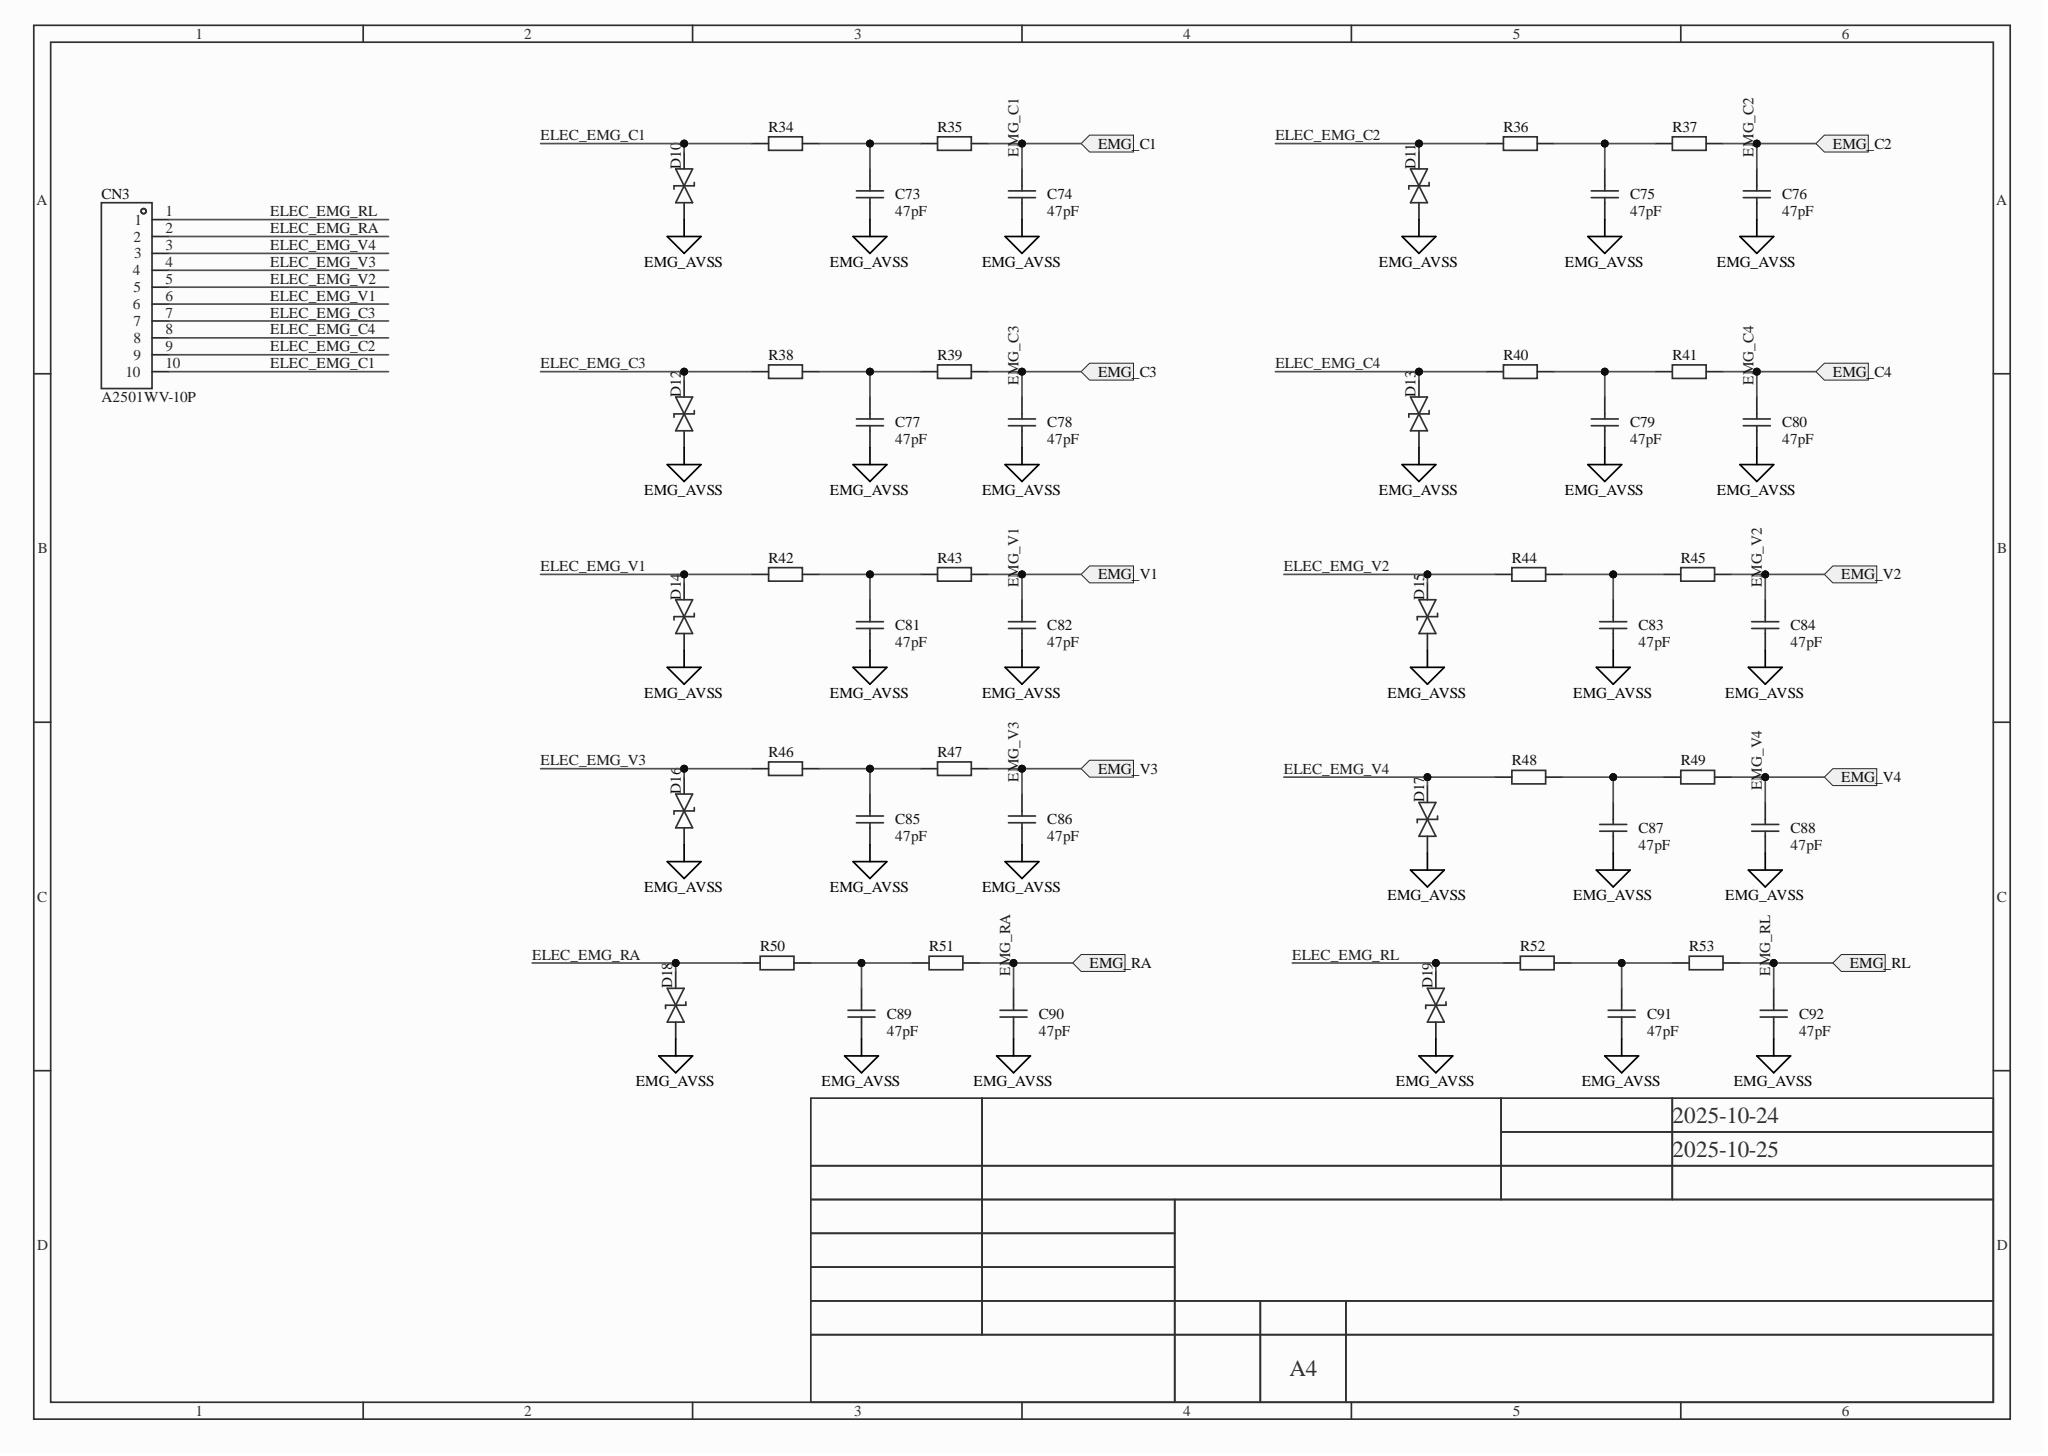Circuit board | Altium Designer | 212 parts | 123 nets | one sheet of the schematic
Parts on this sheet (reference | value | footprint):
C73 | 47pF | C0402
C74 | 47pF | C0402
C75 | 47pF | C0402
C76 | 47pF | C0402
C77 | 47pF | C0402
C78 | 47pF | C0402
C79 | 47pF | C0402
C80 | 47pF | C0402
C81 | 47pF | C0402
C82 | 47pF | C0402
C83 | 47pF | C0402
C84 | 47pF | C0402
C85 | 47pF | C0402
C86 | 47pF | C0402
C87 | 47pF | C0402
C88 | 47pF | C0402
C89 | 47pF | C0402
C90 | 47pF | C0402
C91 | 47pF | C0402
C92 | 47pF | C0402
CN3 | A2501WV-10P | CONN-TH_A2501WV-10P
D10 | TPD1E10B06DPYR-TP | X1-DFN1006-2_L1.0-W0.6-BI
D11 | TPD1E10B06DPYR-TP | X1-DFN1006-2_L1.0-W0.6-BI
D12 | TPD1E10B06DPYR-TP | X1-DFN1006-2_L1.0-W0.6-BI
D13 | TPD1E10B06DPYR-TP | X1-DFN1006-2_L1.0-W0.6-BI
D14 | TPD1E10B06DPYR-TP | X1-DFN1006-2_L1.0-W0.6-BI
D15 | TPD1E10B06DPYR-TP | X1-DFN1006-2_L1.0-W0.6-BI
D16 | TPD1E10B06DPYR-TP | X1-DFN1006-2_L1.0-W0.6-BI
D17 | TPD1E10B06DPYR-TP | X1-DFN1006-2_L1.0-W0.6-BI
D18 | TPD1E10B06DPYR-TP | X1-DFN1006-2_L1.0-W0.6-BI
D19 | TPD1E10B06DPYR-TP | X1-DFN1006-2_L1.0-W0.6-BI
R34 | R0402
R35 | R0402
R36 | R0402
R37 | R0402
R38 | R0402
R39 | R0402
R40 | R0402
R41 | R0402
R42 | R0402
R43 | R0402
R44 | R0402
R45 | R0402
R46 | R0402
R47 | R0402
R48 | R0402
R49 | R0402
R50 | R0402
R51 | R0402
R52 | R0402
R53 | R0402
Nets of these parts (net: part-pin ...):
NetC91_2: C91-2 R52-2 R53-1
NetC89_2: C89-2 R50-2 R51-1
NetC87_2: C87-2 R48-2 R49-1
NetC85_2: C85-2 R46-2 R47-1
NetC83_2: C83-2 R44-2 R45-1
NetC81_2: C81-2 R42-2 R43-1
NetC79_2: C79-2 R40-2 R41-1
NetC77_2: C77-2 R38-2 R39-1
NetC75_2: C75-2 R36-2 R37-1
NetC73_2: C73-2 R34-2 R35-1
EMG_V4: C88-2 R49-2
EMG_V3: C86-2 R47-2
EMG_V2: C84-2 R45-2
EMG_V1: C82-2 R43-2
EMG_RL: C92-2 R53-2
EMG_RA: C90-2 R51-2
EMG_C4: C80-2 R41-2
EMG_C3: C78-2 R39-2
EMG_C2: C76-2 R37-2
EMG_C1: C74-2 R35-2
EMG_AVSS1: C73-1 C74-1 C75-1 C76-1 C77-1 C78-1 C79-1 C80-1 C81-1 C82-1 C83-1 C84-1 C85-1 C86-1 C87-1 C88-1 C89-1 C90-1 C91-1 C92-1 D10-1 D11-1 D12-1 D13-1 D14-1 D15-1 D16-1 D17-1 D18-1 D19-1
ELEC_EMG_V4: CN3-3 D17-2 R48-1
ELEC_EMG_V3: CN3-4 D16-2 R46-1
ELEC_EMG_V2: CN3-5 D15-2 R44-1
ELEC_EMG_V1: CN3-6 D14-2 R42-1
ELEC_EMG_RL: CN3-1 D19-2 R52-1
ELEC_EMG_RA: CN3-2 D18-2 R50-1
ELEC_EMG_C4: CN3-8 D13-2 R40-1
ELEC_EMG_C3: CN3-7 D12-2 R38-1
ELEC_EMG_C2: CN3-9 D11-2 R36-1
ELEC_EMG_C1: CN3-10 D10-2 R34-1